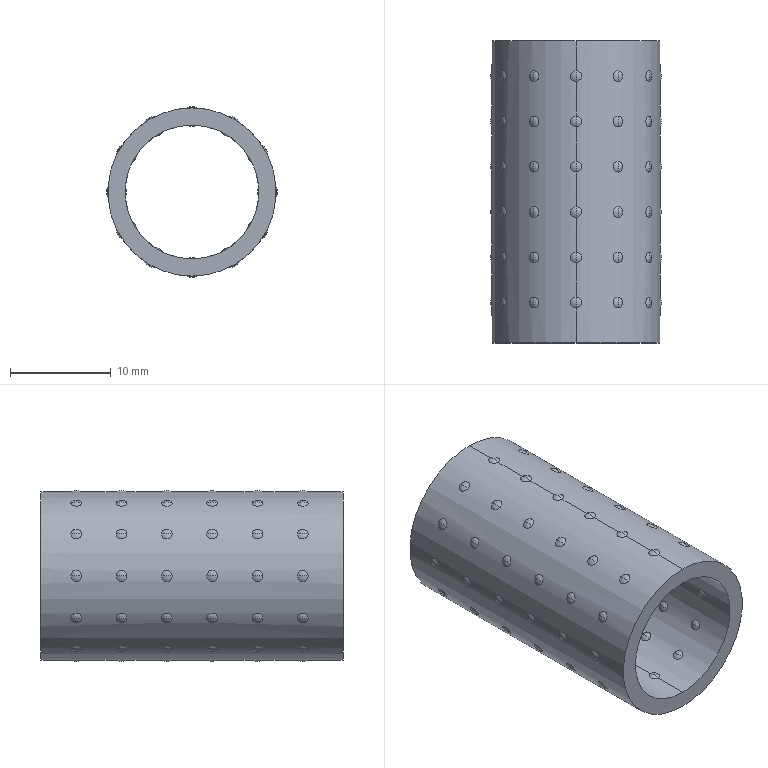Part | SolidWorks | features CirPattern 2, LPattern 2, RefAxis 2, Extrusion 1, ICE 1, Revolution 1 | 1 solid | 294 faces | box 17 x 30 x 17 mm | volume 2413 mm3 | sphere 288 | cylinder 4 | plane 2 | commonest cylinder face diameters 13.3 x2 16.7 x2